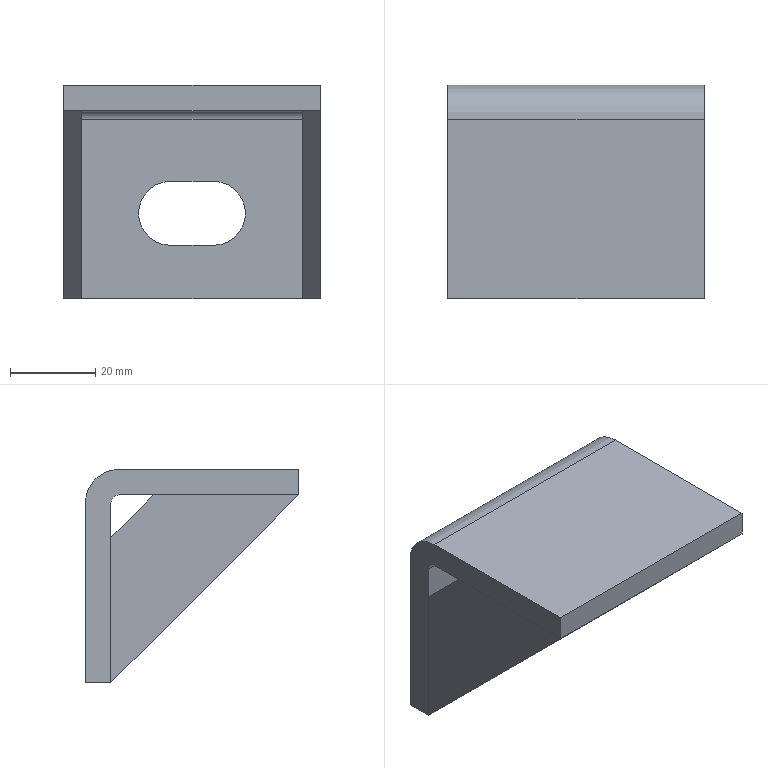Part | STEP file | HL4GZ-1.581.018 (tank bottom mounting seat weldment) | 3 solids | 26 faces | box 60 x 50 x 50 mm | volume 38451 mm3 | plane 22 | cylinder 4 | commonest cylinder face diameters 15 x2 4 x1 16 x1